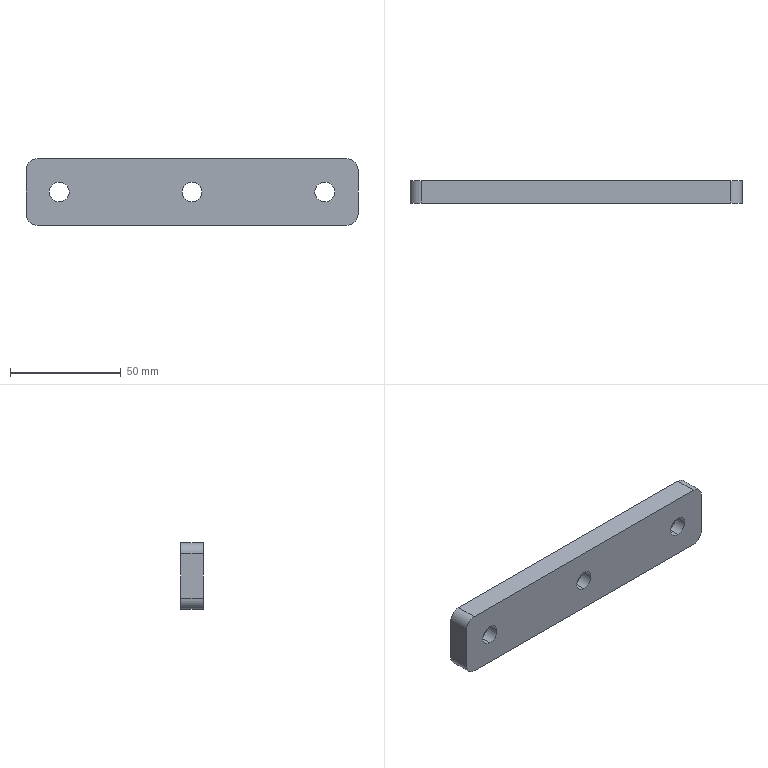Part | SolidWorks | features LPattern 2, Extrusion 1, Fillet 1, HoleWzd 1, ICE 1 | 1 solid | 22 faces | box 150 x 10 x 30 mm | volume 41843 mm3 | cylinder 10 | cone 6 | plane 6 | commonest cylinder face diameters 9 x6 10 x4
STEP:
#1=CARTESIAN_POINT('',(75.,5.7,-19.5));
#2=VERTEX_POINT('',#1);
#3=CARTESIAN_POINT('',(75.,5.7,-10.5));
#4=VERTEX_POINT('',#3);
#5=CARTESIAN_POINT('',(75.,5.7,-15.));
#6=DIRECTION('',(0.,1.,0.));
#7=DIRECTION('',(0.,0.,1.));
#8=AXIS2_PLACEMENT_3D('',#5,#6,#7);
#9=CIRCLE('',#8,4.5);
#10=EDGE_CURVE('',#2,#4,#9,.T.);
#11=ORIENTED_EDGE('',*,*,#10,.F.);
#12=CARTESIAN_POINT('',(75.,10.,-23.8));
#13=VERTEX_POINT('',#12);
#14=CARTESIAN_POINT('',(75.,10.,-23.8));
#15=DIRECTION('',(0.,0.7071,-0.7071));
#16=VECTOR('',#15,1000.);
#17=LINE('',#14,#16);
#18=EDGE_CURVE('',#2,#13,#17,.T.);
#19=ORIENTED_EDGE('',*,*,#18,.T.);
#20=CARTESIAN_POINT('',(75.,10.,-6.2));
#21=VERTEX_POINT('',#20);
#22=CARTESIAN_POINT('',(75.,10.,-15.));
#23=DIRECTION('',(0.,1.,0.));
#24=DIRECTION('',(0.,0.,1.));
#25=AXIS2_PLACEMENT_3D('',#22,#23,#24);
#26=CIRCLE('',#25,8.8);
#27=EDGE_CURVE('',#13,#21,#26,.T.);
#28=ORIENTED_EDGE('',*,*,#27,.T.);
#29=CARTESIAN_POINT('',(75.,10.,-6.2));
#30=DIRECTION('',(0.,0.7071,0.7071));
#31=VECTOR('',#30,1000.);
#32=LINE('',#29,#31);
#33=EDGE_CURVE('',#4,#21,#32,.T.);
#34=ORIENTED_EDGE('',*,*,#33,.F.);
#35=EDGE_LOOP('',(#11,#19,#28,#34));
#36=FACE_OUTER_BOUND('',#35,.T.);
#37=CARTESIAN_POINT('',(75.,10.,-15.));
#38=DIRECTION('',(0.,1.,0.));
#39=DIRECTION('',(0.,0.,1.));
#40=AXIS2_PLACEMENT_3D('',#37,#38,#39);
#41=CONICAL_SURFACE('',#40,8.8,0.7854);
#42=ADVANCED_FACE('',(#36),#41,.F.);
#43=CARTESIAN_POINT('',(75.,0.,-10.5));
#44=VERTEX_POINT('',#43);
#45=CARTESIAN_POINT('',(75.,0.,-19.5));
#46=VERTEX_POINT('',#45);
#47=CARTESIAN_POINT('',(75.,0.,-15.));
#48=DIRECTION('',(0.,-1.,0.));
#49=DIRECTION('',(0.,0.,-1.));
#50=AXIS2_PLACEMENT_3D('',#47,#48,#49);
#51=CIRCLE('',#50,4.5);
#52=EDGE_CURVE('',#44,#46,#51,.T.);
#53=ORIENTED_EDGE('',*,*,#52,.T.);
#54=CARTESIAN_POINT('',(75.,10.,-19.5));
#55=DIRECTION('',(0.,1.,0.));
#56=VECTOR('',#55,1000.);
#57=LINE('',#54,#56);
#58=EDGE_CURVE('',#46,#2,#57,.T.);
#59=ORIENTED_EDGE('',*,*,#58,.T.);
#60=ORIENTED_EDGE('',*,*,#10,.T.);
#61=CARTESIAN_POINT('',(75.,10.,-10.5));
#62=DIRECTION('',(0.,1.,0.));
#63=VECTOR('',#62,1000.);
#64=LINE('',#61,#63);
#65=EDGE_CURVE('',#44,#4,#64,.T.);
#66=ORIENTED_EDGE('',*,*,#65,.F.);
#67=EDGE_LOOP('',(#53,#59,#60,#66));
#68=FACE_OUTER_BOUND('',#67,.T.);
#69=CARTESIAN_POINT('',(75.,10.,-15.));
#70=DIRECTION('',(0.,1.,0.));
#71=DIRECTION('',(0.,0.,1.));
#72=AXIS2_PLACEMENT_3D('',#69,#70,#71);
#73=CYLINDRICAL_SURFACE('',#72,4.5);
#74=ADVANCED_FACE('',(#68),#73,.F.);
#75=CARTESIAN_POINT('',(15.,5.7,-19.5));
#76=VERTEX_POINT('',#75);
#77=CARTESIAN_POINT('',(15.,5.7,-10.5));
#78=VERTEX_POINT('',#77);
#79=CARTESIAN_POINT('',(15.,5.7,-15.));
#80=DIRECTION('',(0.,1.,0.));
#81=DIRECTION('',(0.,0.,1.));
#82=AXIS2_PLACEMENT_3D('',#79,#80,#81);
#83=CIRCLE('',#82,4.5);
#84=EDGE_CURVE('',#76,#78,#83,.T.);
#85=ORIENTED_EDGE('',*,*,#84,.F.);
#86=CARTESIAN_POINT('',(15.,10.,-23.8));
#87=VERTEX_POINT('',#86);
#88=CARTESIAN_POINT('',(15.,10.,-23.8));
#89=DIRECTION('',(0.,0.7071,-0.7071));
#90=VECTOR('',#89,1000.);
#91=LINE('',#88,#90);
#92=EDGE_CURVE('',#76,#87,#91,.T.);
#93=ORIENTED_EDGE('',*,*,#92,.T.);
#94=CARTESIAN_POINT('',(15.,10.,-6.2));
#95=VERTEX_POINT('',#94);
#96=CARTESIAN_POINT('',(15.,10.,-15.));
#97=DIRECTION('',(0.,1.,0.));
#98=DIRECTION('',(0.,0.,1.));
#99=AXIS2_PLACEMENT_3D('',#96,#97,#98);
#100=CIRCLE('',#99,8.8);
#101=EDGE_CURVE('',#87,#95,#100,.T.);
#102=ORIENTED_EDGE('',*,*,#101,.T.);
#103=CARTESIAN_POINT('',(15.,10.,-6.2));
#104=DIRECTION('',(0.,0.7071,0.7071));
#105=VECTOR('',#104,1000.);
#106=LINE('',#103,#105);
#107=EDGE_CURVE('',#78,#95,#106,.T.);
#108=ORIENTED_EDGE('',*,*,#107,.F.);
#109=EDGE_LOOP('',(#85,#93,#102,#108));
#110=FACE_OUTER_BOUND('',#109,.T.);
#111=CARTESIAN_POINT('',(15.,10.,-15.));
#112=DIRECTION('',(0.,1.,0.));
#113=DIRECTION('',(0.,0.,1.));
#114=AXIS2_PLACEMENT_3D('',#111,#112,#113);
#115=CONICAL_SURFACE('',#114,8.8,0.7854);
#116=ADVANCED_FACE('',(#110),#115,.F.);
#117=CARTESIAN_POINT('',(15.,0.,-10.5));
#118=VERTEX_POINT('',#117);
#119=CARTESIAN_POINT('',(15.,0.,-19.5));
#120=VERTEX_POINT('',#119);
#121=CARTESIAN_POINT('',(15.,0.,-15.));
#122=DIRECTION('',(0.,-1.,0.));
#123=DIRECTION('',(0.,0.,-1.));
#124=AXIS2_PLACEMENT_3D('',#121,#122,#123);
#125=CIRCLE('',#124,4.5);
#126=EDGE_CURVE('',#118,#120,#125,.T.);
#127=ORIENTED_EDGE('',*,*,#126,.T.);
#128=CARTESIAN_POINT('',(15.,10.,-19.5));
#129=DIRECTION('',(0.,1.,0.));
#130=VECTOR('',#129,1000.);
#131=LINE('',#128,#130);
#132=EDGE_CURVE('',#120,#76,#131,.T.);
#133=ORIENTED_EDGE('',*,*,#132,.T.);
#134=ORIENTED_EDGE('',*,*,#84,.T.);
#135=CARTESIAN_POINT('',(15.,10.,-10.5));
#136=DIRECTION('',(0.,1.,0.));
#137=VECTOR('',#136,1000.);
#138=LINE('',#135,#137);
#139=EDGE_CURVE('',#118,#78,#138,.T.);
#140=ORIENTED_EDGE('',*,*,#139,.F.);
#141=EDGE_LOOP('',(#127,#133,#134,#140));
#142=FACE_OUTER_BOUND('',#141,.T.);
#143=CARTESIAN_POINT('',(15.,10.,-15.));
#144=DIRECTION('',(0.,1.,0.));
#145=DIRECTION('',(0.,0.,1.));
#146=AXIS2_PLACEMENT_3D('',#143,#144,#145);
#147=CYLINDRICAL_SURFACE('',#146,4.5);
#148=ADVANCED_FACE('',(#142),#147,.F.);
#149=CARTESIAN_POINT('',(135.,5.7,-19.5));
#150=VERTEX_POINT('',#149);
#151=CARTESIAN_POINT('',(135.,5.7,-10.5));
#152=VERTEX_POINT('',#151);
#153=CARTESIAN_POINT('',(135.,5.7,-15.));
#154=DIRECTION('',(0.,1.,0.));
#155=DIRECTION('',(0.,0.,1.));
#156=AXIS2_PLACEMENT_3D('',#153,#154,#155);
#157=CIRCLE('',#156,4.5);
#158=EDGE_CURVE('',#150,#152,#157,.T.);
#159=ORIENTED_EDGE('',*,*,#158,.F.);
#160=CARTESIAN_POINT('',(135.,10.,-23.8));
#161=VERTEX_POINT('',#160);
#162=CARTESIAN_POINT('',(135.,10.,-23.8));
#163=DIRECTION('',(0.,0.7071,-0.7071));
#164=VECTOR('',#163,1000.);
#165=LINE('',#162,#164);
#166=EDGE_CURVE('',#150,#161,#165,.T.);
#167=ORIENTED_EDGE('',*,*,#166,.T.);
#168=CARTESIAN_POINT('',(135.,10.,-6.2));
#169=VERTEX_POINT('',#168);
#170=CARTESIAN_POINT('',(135.,10.,-15.));
#171=DIRECTION('',(0.,1.,0.));
#172=DIRECTION('',(0.,0.,1.));
#173=AXIS2_PLACEMENT_3D('',#170,#171,#172);
#174=CIRCLE('',#173,8.8);
#175=EDGE_CURVE('',#161,#169,#174,.T.);
#176=ORIENTED_EDGE('',*,*,#175,.T.);
#177=CARTESIAN_POINT('',(135.,10.,-6.2));
#178=DIRECTION('',(0.,0.7071,0.7071));
#179=VECTOR('',#178,1000.);
#180=LINE('',#177,#179);
#181=EDGE_CURVE('',#152,#169,#180,.T.);
#182=ORIENTED_EDGE('',*,*,#181,.F.);
#183=EDGE_LOOP('',(#159,#167,#176,#182));
#184=FACE_OUTER_BOUND('',#183,.T.);
#185=CARTESIAN_POINT('',(135.,10.,-15.));
#186=DIRECTION('',(0.,1.,0.));
#187=DIRECTION('',(0.,0.,1.));
#188=AXIS2_PLACEMENT_3D('',#185,#186,#187);
#189=CONICAL_SURFACE('',#188,8.8,0.7854);
#190=ADVANCED_FACE('',(#184),#189,.F.);
#191=CARTESIAN_POINT('',(135.,0.,-10.5));
#192=VERTEX_POINT('',#191);
#193=CARTESIAN_POINT('',(135.,0.,-19.5));
#194=VERTEX_POINT('',#193);
#195=CARTESIAN_POINT('',(135.,0.,-15.));
#196=DIRECTION('',(0.,-1.,0.));
#197=DIRECTION('',(0.,0.,-1.));
#198=AXIS2_PLACEMENT_3D('',#195,#196,#197);
#199=CIRCLE('',#198,4.5);
#200=EDGE_CURVE('',#192,#194,#199,.T.);
#201=ORIENTED_EDGE('',*,*,#200,.T.);
#202=CARTESIAN_POINT('',(135.,10.,-19.5));
#203=DIRECTION('',(0.,1.,0.));
#204=VECTOR('',#203,1000.);
#205=LINE('',#202,#204);
#206=EDGE_CURVE('',#194,#150,#205,.T.);
#207=ORIENTED_EDGE('',*,*,#206,.T.);
#208=ORIENTED_EDGE('',*,*,#158,.T.);
#209=CARTESIAN_POINT('',(135.,10.,-10.5));
#210=DIRECTION('',(0.,1.,0.));
#211=VECTOR('',#210,1000.);
#212=LINE('',#209,#211);
#213=EDGE_CURVE('',#192,#152,#212,.T.);
#214=ORIENTED_EDGE('',*,*,#213,.F.);
#215=EDGE_LOOP('',(#201,#207,#208,#214));
#216=FACE_OUTER_BOUND('',#215,.T.);
#217=CARTESIAN_POINT('',(135.,10.,-15.));
#218=DIRECTION('',(0.,1.,0.));
#219=DIRECTION('',(0.,0.,1.));
#220=AXIS2_PLACEMENT_3D('',#217,#218,#219);
#221=CYLINDRICAL_SURFACE('',#220,4.5);
#222=ADVANCED_FACE('',(#216),#221,.F.);
#223=CARTESIAN_POINT('',(0.,10.,-25.));
#224=VERTEX_POINT('',#223);
#225=CARTESIAN_POINT('',(0.,10.,-5.));
#226=VERTEX_POINT('',#225);
#227=CARTESIAN_POINT('',(0.,10.,0.));
#228=DIRECTION('',(0.,0.,1.));
#229=VECTOR('',#228,1000.);
#230=LINE('',#227,#229);
#231=EDGE_CURVE('',#224,#226,#230,.T.);
#232=ORIENTED_EDGE('',*,*,#231,.F.);
#233=CARTESIAN_POINT('',(0.,0.,-25.));
#234=VERTEX_POINT('',#233);
#235=CARTESIAN_POINT('',(0.,10.,-25.));
#236=DIRECTION('',(0.,-1.,0.));
#237=VECTOR('',#236,1000.);
#238=LINE('',#235,#237);
#239=EDGE_CURVE('',#224,#234,#238,.T.);
#240=ORIENTED_EDGE('',*,*,#239,.T.);
#241=CARTESIAN_POINT('',(0.,0.,-5.));
#242=VERTEX_POINT('',#241);
#243=CARTESIAN_POINT('',(0.,0.,0.));
#244=DIRECTION('',(0.,0.,1.));
#245=VECTOR('',#244,1000.);
#246=LINE('',#243,#245);
#247=EDGE_CURVE('',#234,#242,#246,.T.);
#248=ORIENTED_EDGE('',*,*,#247,.T.);
#249=CARTESIAN_POINT('',(0.,10.,-5.));
#250=DIRECTION('',(0.,1.,0.));
#251=VECTOR('',#250,1000.);
#252=LINE('',#249,#251);
#253=EDGE_CURVE('',#242,#226,#252,.T.);
#254=ORIENTED_EDGE('',*,*,#253,.T.);
#255=EDGE_LOOP('',(#232,#240,#248,#254));
#256=FACE_OUTER_BOUND('',#255,.T.);
#257=CARTESIAN_POINT('',(0.,10.,0.));
#258=DIRECTION('',(1.,0.,0.));
#259=DIRECTION('',(0.,0.,-1.));
#260=AXIS2_PLACEMENT_3D('',#257,#258,#259);
#261=PLANE('',#260);
#262=ADVANCED_FACE('',(#256),#261,.F.);
#263=CARTESIAN_POINT('',(5.,0.,0.));
#264=VERTEX_POINT('',#263);
#265=CARTESIAN_POINT('',(145.,0.,0.));
#266=VERTEX_POINT('',#265);
#267=CARTESIAN_POINT('',(0.,0.,0.));
#268=DIRECTION('',(1.,0.,0.));
#269=VECTOR('',#268,1000.);
#270=LINE('',#267,#269);
#271=EDGE_CURVE('',#264,#266,#270,.T.);
#272=ORIENTED_EDGE('',*,*,#271,.T.);
#273=CARTESIAN_POINT('',(145.,10.,0.));
#274=VERTEX_POINT('',#273);
#275=CARTESIAN_POINT('',(145.,10.,0.));
#276=DIRECTION('',(0.,1.,0.));
#277=VECTOR('',#276,1000.);
#278=LINE('',#275,#277);
#279=EDGE_CURVE('',#266,#274,#278,.T.);
#280=ORIENTED_EDGE('',*,*,#279,.T.);
#281=CARTESIAN_POINT('',(5.,10.,0.));
#282=VERTEX_POINT('',#281);
#283=CARTESIAN_POINT('',(0.,10.,0.));
#284=DIRECTION('',(1.,0.,0.));
#285=VECTOR('',#284,1000.);
#286=LINE('',#283,#285);
#287=EDGE_CURVE('',#282,#274,#286,.T.);
#288=ORIENTED_EDGE('',*,*,#287,.F.);
#289=CARTESIAN_POINT('',(5.,10.,0.));
#290=DIRECTION('',(0.,-1.,0.));
#291=VECTOR('',#290,1000.);
#292=LINE('',#289,#291);
#293=EDGE_CURVE('',#282,#264,#292,.T.);
#294=ORIENTED_EDGE('',*,*,#293,.T.);
#295=EDGE_LOOP('',(#272,#280,#288,#294));
#296=FACE_OUTER_BOUND('',#295,.T.);
#297=CARTESIAN_POINT('',(0.,10.,0.));
#298=DIRECTION('',(0.,0.,-1.));
#299=DIRECTION('',(-1.,0.,0.));
#300=AXIS2_PLACEMENT_3D('',#297,#298,#299);
#301=PLANE('',#300);
#302=ADVANCED_FACE('',(#296),#301,.F.);
#303=CARTESIAN_POINT('',(150.,0.,-5.));
#304=VERTEX_POINT('',#303);
#305=CARTESIAN_POINT('',(150.,0.,-25.));
#306=VERTEX_POINT('',#305);
#307=CARTESIAN_POINT('',(150.,0.,0.));
#308=DIRECTION('',(0.,0.,-1.));
#309=VECTOR('',#308,1000.);
#310=LINE('',#307,#309);
#311=EDGE_CURVE('',#304,#306,#310,.T.);
#312=ORIENTED_EDGE('',*,*,#311,.T.);
#313=CARTESIAN_POINT('',(150.,10.,-25.));
#314=VERTEX_POINT('',#313);
#315=CARTESIAN_POINT('',(150.,10.,-25.));
#316=DIRECTION('',(0.,1.,0.));
#317=VECTOR('',#316,1000.);
#318=LINE('',#315,#317);
#319=EDGE_CURVE('',#306,#314,#318,.T.);
#320=ORIENTED_EDGE('',*,*,#319,.T.);
#321=CARTESIAN_POINT('',(150.,10.,-5.));
#322=VERTEX_POINT('',#321);
#323=CARTESIAN_POINT('',(150.,10.,0.));
#324=DIRECTION('',(0.,0.,-1.));
#325=VECTOR('',#324,1000.);
#326=LINE('',#323,#325);
#327=EDGE_CURVE('',#322,#314,#326,.T.);
#328=ORIENTED_EDGE('',*,*,#327,.F.);
#329=CARTESIAN_POINT('',(150.,10.,-5.));
#330=DIRECTION('',(0.,-1.,0.));
#331=VECTOR('',#330,1000.);
#332=LINE('',#329,#331);
#333=EDGE_CURVE('',#322,#304,#332,.T.);
#334=ORIENTED_EDGE('',*,*,#333,.T.);
#335=EDGE_LOOP('',(#312,#320,#328,#334));
#336=FACE_OUTER_BOUND('',#335,.T.);
#337=CARTESIAN_POINT('',(150.,10.,0.));
#338=DIRECTION('',(-1.,0.,0.));
#339=DIRECTION('',(0.,0.,1.));
#340=AXIS2_PLACEMENT_3D('',#337,#338,#339);
#341=PLANE('',#340);
#342=ADVANCED_FACE('',(#336),#341,.F.);
#343=CARTESIAN_POINT('',(145.,0.,-30.));
#344=VERTEX_POINT('',#343);
#345=CARTESIAN_POINT('',(5.,0.,-30.));
#346=VERTEX_POINT('',#345);
#347=CARTESIAN_POINT('',(0.,0.,-30.));
#348=DIRECTION('',(-1.,0.,0.));
#349=VECTOR('',#348,1000.);
#350=LINE('',#347,#349);
#351=EDGE_CURVE('',#344,#346,#350,.T.);
#352=ORIENTED_EDGE('',*,*,#351,.T.);
#353=CARTESIAN_POINT('',(5.,10.,-30.));
#354=VERTEX_POINT('',#353);
#355=CARTESIAN_POINT('',(5.,10.,-30.));
#356=DIRECTION('',(0.,1.,0.));
#357=VECTOR('',#356,1000.);
#358=LINE('',#355,#357);
#359=EDGE_CURVE('',#346,#354,#358,.T.);
#360=ORIENTED_EDGE('',*,*,#359,.T.);
#361=CARTESIAN_POINT('',(145.,10.,-30.));
#362=VERTEX_POINT('',#361);
#363=CARTESIAN_POINT('',(0.,10.,-30.));
#364=DIRECTION('',(-1.,0.,0.));
#365=VECTOR('',#364,1000.);
#366=LINE('',#363,#365);
#367=EDGE_CURVE('',#362,#354,#366,.T.);
#368=ORIENTED_EDGE('',*,*,#367,.F.);
#369=CARTESIAN_POINT('',(145.,10.,-30.));
#370=DIRECTION('',(0.,-1.,0.));
#371=VECTOR('',#370,1000.);
#372=LINE('',#369,#371);
#373=EDGE_CURVE('',#362,#344,#372,.T.);
#374=ORIENTED_EDGE('',*,*,#373,.T.);
#375=EDGE_LOOP('',(#352,#360,#368,#374));
#376=FACE_OUTER_BOUND('',#375,.T.);
#377=CARTESIAN_POINT('',(0.,10.,-30.));
#378=DIRECTION('',(0.,0.,1.));
#379=DIRECTION('',(1.,0.,0.));
#380=AXIS2_PLACEMENT_3D('',#377,#378,#379);
#381=PLANE('',#380);
#382=ADVANCED_FACE('',(#376),#381,.F.);
#383=CARTESIAN_POINT('',(75.,10.,-15.));
#384=DIRECTION('',(0.,1.,0.));
#385=DIRECTION('',(0.,0.,1.));
#386=AXIS2_PLACEMENT_3D('',#383,#384,#385);
#387=CIRCLE('',#386,8.8);
#388=EDGE_CURVE('',#21,#13,#387,.T.);
#389=ORIENTED_EDGE('',*,*,#388,.F.);
#390=ORIENTED_EDGE('',*,*,#27,.F.);
#391=EDGE_LOOP('',(#389,#390));
#392=FACE_BOUND('',#391,.T.);
#393=CARTESIAN_POINT('',(15.,10.,-15.));
#394=DIRECTION('',(0.,1.,0.));
#395=DIRECTION('',(0.,0.,1.));
#396=AXIS2_PLACEMENT_3D('',#393,#394,#395);
#397=CIRCLE('',#396,8.8);
#398=EDGE_CURVE('',#95,#87,#397,.T.);
#399=ORIENTED_EDGE('',*,*,#398,.F.);
#400=ORIENTED_EDGE('',*,*,#101,.F.);
#401=EDGE_LOOP('',(#399,#400));
#402=FACE_BOUND('',#401,.T.);
#403=CARTESIAN_POINT('',(135.,10.,-15.));
#404=DIRECTION('',(0.,1.,0.));
#405=DIRECTION('',(0.,0.,1.));
#406=AXIS2_PLACEMENT_3D('',#403,#404,#405);
#407=CIRCLE('',#406,8.8);
#408=EDGE_CURVE('',#169,#161,#407,.T.);
#409=ORIENTED_EDGE('',*,*,#408,.F.);
#410=ORIENTED_EDGE('',*,*,#175,.F.);
#411=EDGE_LOOP('',(#409,#410));
#412=FACE_BOUND('',#411,.T.);
#413=ORIENTED_EDGE('',*,*,#367,.T.);
#414=CARTESIAN_POINT('',(5.,10.,-25.));
#415=DIRECTION('',(0.,1.,0.));
#416=DIRECTION('',(0.,0.,-1.));
#417=AXIS2_PLACEMENT_3D('',#414,#415,#416);
#418=CIRCLE('',#417,5.);
#419=EDGE_CURVE('',#354,#224,#418,.T.);
#420=ORIENTED_EDGE('',*,*,#419,.T.);
#421=ORIENTED_EDGE('',*,*,#231,.T.);
#422=CARTESIAN_POINT('',(5.,10.,-5.));
#423=DIRECTION('',(0.,1.,0.));
#424=DIRECTION('',(0.,0.,-1.));
#425=AXIS2_PLACEMENT_3D('',#422,#423,#424);
#426=CIRCLE('',#425,5.);
#427=EDGE_CURVE('',#226,#282,#426,.T.);
#428=ORIENTED_EDGE('',*,*,#427,.T.);
#429=ORIENTED_EDGE('',*,*,#287,.T.);
#430=CARTESIAN_POINT('',(145.,10.,-5.));
#431=DIRECTION('',(0.,1.,0.));
#432=DIRECTION('',(0.,0.,-1.));
#433=AXIS2_PLACEMENT_3D('',#430,#431,#432);
#434=CIRCLE('',#433,5.);
#435=EDGE_CURVE('',#274,#322,#434,.T.);
#436=ORIENTED_EDGE('',*,*,#435,.T.);
#437=ORIENTED_EDGE('',*,*,#327,.T.);
#438=CARTESIAN_POINT('',(145.,10.,-25.));
#439=DIRECTION('',(0.,1.,0.));
#440=DIRECTION('',(0.,0.,-1.));
#441=AXIS2_PLACEMENT_3D('',#438,#439,#440);
#442=CIRCLE('',#441,5.);
#443=EDGE_CURVE('',#314,#362,#442,.T.);
#444=ORIENTED_EDGE('',*,*,#443,.T.);
#445=EDGE_LOOP('',(#413,#420,#421,#428,#429,#436,#437,#444));
#446=FACE_OUTER_BOUND('',#445,.T.);
#447=CARTESIAN_POINT('',(0.,10.,0.));
#448=DIRECTION('',(0.,-1.,0.));
#449=DIRECTION('',(0.,0.,-1.));
#450=AXIS2_PLACEMENT_3D('',#447,#448,#449);
#451=PLANE('',#450);
#452=ADVANCED_FACE('',(#392,#402,#412,#446),#451,.F.);
#453=ORIENTED_EDGE('',*,*,#52,.F.);
#454=CARTESIAN_POINT('',(75.,0.,-15.));
#455=DIRECTION('',(0.,-1.,0.));
#456=DIRECTION('',(0.,0.,-1.));
#457=AXIS2_PLACEMENT_3D('',#454,#455,#456);
#458=CIRCLE('',#457,4.5);
#459=EDGE_CURVE('',#46,#44,#458,.T.);
#460=ORIENTED_EDGE('',*,*,#459,.F.);
#461=EDGE_LOOP('',(#453,#460));
#462=FACE_BOUND('',#461,.T.);
#463=ORIENTED_EDGE('',*,*,#126,.F.);
#464=CARTESIAN_POINT('',(15.,0.,-15.));
#465=DIRECTION('',(0.,-1.,0.));
#466=DIRECTION('',(0.,0.,-1.));
#467=AXIS2_PLACEMENT_3D('',#464,#465,#466);
#468=CIRCLE('',#467,4.5);
#469=EDGE_CURVE('',#120,#118,#468,.T.);
#470=ORIENTED_EDGE('',*,*,#469,.F.);
#471=EDGE_LOOP('',(#463,#470));
#472=FACE_BOUND('',#471,.T.);
#473=ORIENTED_EDGE('',*,*,#200,.F.);
#474=CARTESIAN_POINT('',(135.,0.,-15.));
#475=DIRECTION('',(0.,-1.,0.));
#476=DIRECTION('',(0.,0.,-1.));
#477=AXIS2_PLACEMENT_3D('',#474,#475,#476);
#478=CIRCLE('',#477,4.5);
#479=EDGE_CURVE('',#194,#192,#478,.T.);
#480=ORIENTED_EDGE('',*,*,#479,.F.);
#481=EDGE_LOOP('',(#473,#480));
#482=FACE_BOUND('',#481,.T.);
#483=ORIENTED_EDGE('',*,*,#247,.F.);
#484=CARTESIAN_POINT('',(5.,0.,-25.));
#485=DIRECTION('',(0.,-1.,0.));
#486=DIRECTION('',(0.,0.,-1.));
#487=AXIS2_PLACEMENT_3D('',#484,#485,#486);
#488=CIRCLE('',#487,5.);
#489=EDGE_CURVE('',#234,#346,#488,.T.);
#490=ORIENTED_EDGE('',*,*,#489,.T.);
#491=ORIENTED_EDGE('',*,*,#351,.F.);
#492=CARTESIAN_POINT('',(145.,0.,-25.));
#493=DIRECTION('',(0.,-1.,0.));
#494=DIRECTION('',(0.,0.,-1.));
#495=AXIS2_PLACEMENT_3D('',#492,#493,#494);
#496=CIRCLE('',#495,5.);
#497=EDGE_CURVE('',#344,#306,#496,.T.);
#498=ORIENTED_EDGE('',*,*,#497,.T.);
#499=ORIENTED_EDGE('',*,*,#311,.F.);
#500=CARTESIAN_POINT('',(145.,0.,-5.));
#501=DIRECTION('',(0.,-1.,0.));
#502=DIRECTION('',(0.,0.,-1.));
#503=AXIS2_PLACEMENT_3D('',#500,#501,#502);
#504=CIRCLE('',#503,5.);
#505=EDGE_CURVE('',#304,#266,#504,.T.);
#506=ORIENTED_EDGE('',*,*,#505,.T.);
#507=ORIENTED_EDGE('',*,*,#271,.F.);
#508=CARTESIAN_POINT('',(5.,0.,-5.));
#509=DIRECTION('',(0.,-1.,0.));
#510=DIRECTION('',(0.,0.,-1.));
#511=AXIS2_PLACEMENT_3D('',#508,#509,#510);
#512=CIRCLE('',#511,5.);
#513=EDGE_CURVE('',#264,#242,#512,.T.);
#514=ORIENTED_EDGE('',*,*,#513,.T.);
#515=EDGE_LOOP('',(#483,#490,#491,#498,#499,#506,#507,#514));
#516=FACE_OUTER_BOUND('',#515,.T.);
#517=CARTESIAN_POINT('',(0.,0.,0.));
#518=DIRECTION('',(0.,-1.,0.));
#519=DIRECTION('',(0.,0.,-1.));
#520=AXIS2_PLACEMENT_3D('',#517,#518,#519);
#521=PLANE('',#520);
#522=ADVANCED_FACE('',(#462,#472,#482,#516),#521,.T.);
#523=ORIENTED_EDGE('',*,*,#419,.F.);
#524=ORIENTED_EDGE('',*,*,#359,.F.);
#525=ORIENTED_EDGE('',*,*,#489,.F.);
#526=ORIENTED_EDGE('',*,*,#239,.F.);
#527=EDGE_LOOP('',(#523,#524,#525,#526));
#528=FACE_OUTER_BOUND('',#527,.T.);
#529=CARTESIAN_POINT('',(5.,10.,-25.));
#530=DIRECTION('',(0.,-1.,0.));
#531=DIRECTION('',(0.,0.,-1.));
#532=AXIS2_PLACEMENT_3D('',#529,#530,#531);
#533=CYLINDRICAL_SURFACE('',#532,5.);
#534=ADVANCED_FACE('',(#528),#533,.T.);
#535=ORIENTED_EDGE('',*,*,#443,.F.);
#536=ORIENTED_EDGE('',*,*,#319,.F.);
#537=ORIENTED_EDGE('',*,*,#497,.F.);
#538=ORIENTED_EDGE('',*,*,#373,.F.);
#539=EDGE_LOOP('',(#535,#536,#537,#538));
#540=FACE_OUTER_BOUND('',#539,.T.);
#541=CARTESIAN_POINT('',(145.,10.,-25.));
#542=DIRECTION('',(0.,-1.,0.));
#543=DIRECTION('',(0.,0.,-1.));
#544=AXIS2_PLACEMENT_3D('',#541,#542,#543);
#545=CYLINDRICAL_SURFACE('',#544,5.);
#546=ADVANCED_FACE('',(#540),#545,.T.);
#547=ORIENTED_EDGE('',*,*,#435,.F.);
#548=ORIENTED_EDGE('',*,*,#279,.F.);
#549=ORIENTED_EDGE('',*,*,#505,.F.);
#550=ORIENTED_EDGE('',*,*,#333,.F.);
#551=EDGE_LOOP('',(#547,#548,#549,#550));
#552=FACE_OUTER_BOUND('',#551,.T.);
#553=CARTESIAN_POINT('',(145.,10.,-5.));
#554=DIRECTION('',(0.,-1.,0.));
#555=DIRECTION('',(0.,0.,-1.));
#556=AXIS2_PLACEMENT_3D('',#553,#554,#555);
#557=CYLINDRICAL_SURFACE('',#556,5.);
#558=ADVANCED_FACE('',(#552),#557,.T.);
#559=ORIENTED_EDGE('',*,*,#427,.F.);
#560=ORIENTED_EDGE('',*,*,#253,.F.);
#561=ORIENTED_EDGE('',*,*,#513,.F.);
#562=ORIENTED_EDGE('',*,*,#293,.F.);
#563=EDGE_LOOP('',(#559,#560,#561,#562));
#564=FACE_OUTER_BOUND('',#563,.T.);
#565=CARTESIAN_POINT('',(5.,10.,-5.));
#566=DIRECTION('',(0.,-1.,0.));
#567=DIRECTION('',(0.,0.,-1.));
#568=AXIS2_PLACEMENT_3D('',#565,#566,#567);
#569=CYLINDRICAL_SURFACE('',#568,5.);
#570=ADVANCED_FACE('',(#564),#569,.T.);
#571=ORIENTED_EDGE('',*,*,#206,.F.);
#572=ORIENTED_EDGE('',*,*,#479,.T.);
#573=ORIENTED_EDGE('',*,*,#213,.T.);
#574=CARTESIAN_POINT('',(135.,5.7,-15.));
#575=DIRECTION('',(0.,1.,0.));
#576=DIRECTION('',(0.,0.,1.));
#577=AXIS2_PLACEMENT_3D('',#574,#575,#576);
#578=CIRCLE('',#577,4.5);
#579=EDGE_CURVE('',#152,#150,#578,.T.);
#580=ORIENTED_EDGE('',*,*,#579,.T.);
#581=EDGE_LOOP('',(#571,#572,#573,#580));
#582=FACE_OUTER_BOUND('',#581,.T.);
#583=CARTESIAN_POINT('',(135.,10.,-15.));
#584=DIRECTION('',(0.,1.,0.));
#585=DIRECTION('',(0.,0.,1.));
#586=AXIS2_PLACEMENT_3D('',#583,#584,#585);
#587=CYLINDRICAL_SURFACE('',#586,4.5);
#588=ADVANCED_FACE('',(#582),#587,.F.);
#589=ORIENTED_EDGE('',*,*,#166,.F.);
#590=ORIENTED_EDGE('',*,*,#579,.F.);
#591=ORIENTED_EDGE('',*,*,#181,.T.);
#592=ORIENTED_EDGE('',*,*,#408,.T.);
#593=EDGE_LOOP('',(#589,#590,#591,#592));
#594=FACE_OUTER_BOUND('',#593,.T.);
#595=CARTESIAN_POINT('',(135.,10.,-15.));
#596=DIRECTION('',(0.,1.,0.));
#597=DIRECTION('',(0.,0.,1.));
#598=AXIS2_PLACEMENT_3D('',#595,#596,#597);
#599=CONICAL_SURFACE('',#598,8.8,0.7854);
#600=ADVANCED_FACE('',(#594),#599,.F.);
#601=ORIENTED_EDGE('',*,*,#132,.F.);
#602=ORIENTED_EDGE('',*,*,#469,.T.);
#603=ORIENTED_EDGE('',*,*,#139,.T.);
#604=CARTESIAN_POINT('',(15.,5.7,-15.));
#605=DIRECTION('',(0.,1.,0.));
#606=DIRECTION('',(0.,0.,1.));
#607=AXIS2_PLACEMENT_3D('',#604,#605,#606);
#608=CIRCLE('',#607,4.5);
#609=EDGE_CURVE('',#78,#76,#608,.T.);
#610=ORIENTED_EDGE('',*,*,#609,.T.);
#611=EDGE_LOOP('',(#601,#602,#603,#610));
#612=FACE_OUTER_BOUND('',#611,.T.);
#613=CARTESIAN_POINT('',(15.,10.,-15.));
#614=DIRECTION('',(0.,1.,0.));
#615=DIRECTION('',(0.,0.,1.));
#616=AXIS2_PLACEMENT_3D('',#613,#614,#615);
#617=CYLINDRICAL_SURFACE('',#616,4.5);
#618=ADVANCED_FACE('',(#612),#617,.F.);
#619=ORIENTED_EDGE('',*,*,#92,.F.);
#620=ORIENTED_EDGE('',*,*,#609,.F.);
#621=ORIENTED_EDGE('',*,*,#107,.T.);
#622=ORIENTED_EDGE('',*,*,#398,.T.);
#623=EDGE_LOOP('',(#619,#620,#621,#622));
#624=FACE_OUTER_BOUND('',#623,.T.);
#625=CARTESIAN_POINT('',(15.,10.,-15.));
#626=DIRECTION('',(0.,1.,0.));
#627=DIRECTION('',(0.,0.,1.));
#628=AXIS2_PLACEMENT_3D('',#625,#626,#627);
#629=CONICAL_SURFACE('',#628,8.8,0.7854);
#630=ADVANCED_FACE('',(#624),#629,.F.);
#631=ORIENTED_EDGE('',*,*,#58,.F.);
#632=ORIENTED_EDGE('',*,*,#459,.T.);
#633=ORIENTED_EDGE('',*,*,#65,.T.);
#634=CARTESIAN_POINT('',(75.,5.7,-15.));
#635=DIRECTION('',(0.,1.,0.));
#636=DIRECTION('',(0.,0.,1.));
#637=AXIS2_PLACEMENT_3D('',#634,#635,#636);
#638=CIRCLE('',#637,4.5);
#639=EDGE_CURVE('',#4,#2,#638,.T.);
#640=ORIENTED_EDGE('',*,*,#639,.T.);
#641=EDGE_LOOP('',(#631,#632,#633,#640));
#642=FACE_OUTER_BOUND('',#641,.T.);
#643=CARTESIAN_POINT('',(75.,10.,-15.));
#644=DIRECTION('',(0.,1.,0.));
#645=DIRECTION('',(0.,0.,1.));
#646=AXIS2_PLACEMENT_3D('',#643,#644,#645);
#647=CYLINDRICAL_SURFACE('',#646,4.5);
#648=ADVANCED_FACE('',(#642),#647,.F.);
#649=ORIENTED_EDGE('',*,*,#18,.F.);
#650=ORIENTED_EDGE('',*,*,#639,.F.);
#651=ORIENTED_EDGE('',*,*,#33,.T.);
#652=ORIENTED_EDGE('',*,*,#388,.T.);
#653=EDGE_LOOP('',(#649,#650,#651,#652));
#654=FACE_OUTER_BOUND('',#653,.T.);
#655=CARTESIAN_POINT('',(75.,10.,-15.));
#656=DIRECTION('',(0.,1.,0.));
#657=DIRECTION('',(0.,0.,1.));
#658=AXIS2_PLACEMENT_3D('',#655,#656,#657);
#659=CONICAL_SURFACE('',#658,8.8,0.7854);
#660=ADVANCED_FACE('',(#654),#659,.F.);
#661=CLOSED_SHELL('',(#42,#74,#116,#148,#190,#222,#262,#302,#342,#382,#452,#522,#534,#546,#558,#570,#588,#600,#618,#630,#648,#660));
#662=MANIFOLD_SOLID_BREP('',#661);
#663=CARTESIAN_POINT('',(0.,0.,0.));
#664=DIRECTION('',(0.,0.,1.));
#665=DIRECTION('',(1.,0.,0.));
#666=AXIS2_PLACEMENT_3D('',#663,#664,#665);
#667=(LENGTH_UNIT()NAMED_UNIT(*)SI_UNIT(.MILLI.,.METRE.));
#668=UNCERTAINTY_MEASURE_WITH_UNIT(LENGTH_MEASURE(0.00001),#667,'','');
#669=(NAMED_UNIT(*)PLANE_ANGLE_UNIT()SI_UNIT($,.RADIAN.));
#670=(NAMED_UNIT(*)SI_UNIT($,.STERADIAN.)SOLID_ANGLE_UNIT());
#671=(GEOMETRIC_REPRESENTATION_CONTEXT(3)GLOBAL_UNCERTAINTY_ASSIGNED_CONTEXT((#668))GLOBAL_UNIT_ASSIGNED_CONTEXT((#667,#669,#670))REPRESENTATION_CONTEXT('',''));
#672=ADVANCED_BREP_SHAPE_REPRESENTATION('',(#662,#666),#671);